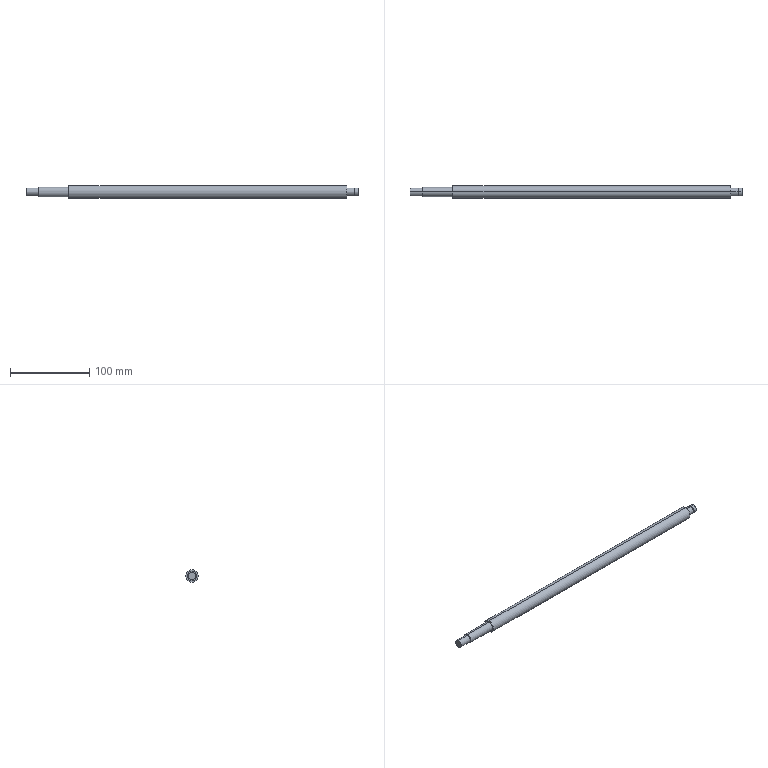Part | STEP file | PN_0033 lead screw 16-5T3 | 1 solid | 19 faces | box 418 x 16 x 16 mm | volume 77018 mm3 | cylinder 12 | plane 7 | commonest cylinder face diameters 10 x6 9.6 x2 12 x2 16 x2
STEP:
#1=CARTESIAN_POINT('',(0.,0.,0.));
#2=DIRECTION('',(0.,0.,1.));
#3=DIRECTION('',(1.,0.,0.));
#4=AXIS2_PLACEMENT_3D('',#1,#2,#3);
#5=CARTESIAN_POINT('',(-3.85,0.,5.));
#6=VERTEX_POINT('',#5);
#7=CARTESIAN_POINT('',(-3.85,0.,-5.));
#8=VERTEX_POINT('',#7);
#9=CARTESIAN_POINT('',(-3.85,0.,0.));
#10=DIRECTION('',(-1.,0.,0.));
#11=DIRECTION('',(0.,0.,-1.));
#12=AXIS2_PLACEMENT_3D('',#9,#10,#11);
#13=CIRCLE('',#12,5.);
#14=CARTESIAN_POINT('',(0.,0.,0.));
#15=DIRECTION('',(1.,0.,0.));
#16=DIRECTION('',(0.,0.,-1.));
#17=AXIS2_PLACEMENT_3D('',#14,#15,#16);
#18=CYLINDRICAL_SURFACE('',#17,5.);
#19=CARTESIAN_POINT('',(6.283,-3.85));
#20=DIRECTION('',(-1.,0.));
#21=VECTOR('',#20,1.);
#22=LINE('',#19,#21);
#23=(GEOMETRIC_REPRESENTATION_CONTEXT(2)PARAMETRIC_REPRESENTATION_CONTEXT()REPRESENTATION_CONTEXT('',''));
#24=DEFINITIONAL_REPRESENTATION('',(#22),#23);
#25=PCURVE('',#18,#24);
#26=CARTESIAN_POINT('',(-3.85,0.,-10.353));
#27=DIRECTION('',(1.,0.,0.));
#28=DIRECTION('',(0.,0.,-1.));
#29=AXIS2_PLACEMENT_3D('',#26,#27,#28);
#30=PLANE('',#29);
#31=CARTESIAN_POINT('',(-5.353,0.));
#32=CARTESIAN_POINT('',(-5.353,-8.66));
#33=CARTESIAN_POINT('',(-12.853,-4.33));
#34=CARTESIAN_POINT('',(-20.353,0.));
#35=CARTESIAN_POINT('',(-12.853,4.33));
#36=CARTESIAN_POINT('',(-5.353,8.66));
#37=CARTESIAN_POINT('',(-5.353,0.));
#38=(BOUNDED_CURVE()B_SPLINE_CURVE(2,(#31,#32,#33,#34,#35,#36,#37),.UNSPECIFIED.,.T.,.F.)B_SPLINE_CURVE_WITH_KNOTS((1,2,2,2,2,1),(-2.094,0.,2.094,4.189,6.283,8.378),.UNSPECIFIED.)CURVE()GEOMETRIC_REPRESENTATION_ITEM()RATIONAL_B_SPLINE_CURVE((1.,0.5,1.,0.5,1.,0.5,1.))REPRESENTATION_ITEM(''));
#39=(GEOMETRIC_REPRESENTATION_CONTEXT(2)PARAMETRIC_REPRESENTATION_CONTEXT()REPRESENTATION_CONTEXT('',''));
#40=DEFINITIONAL_REPRESENTATION('',(#38),#39);
#41=PCURVE('',#30,#40);
#42=SURFACE_CURVE('',#13,(#25,#41),.PCURVE_S1.);
#43=EDGE_CURVE('',#6,#8,#42,.T.);
#44=ORIENTED_EDGE('',*,*,#43,.F.);
#45=CARTESIAN_POINT('',(0.,0.,5.));
#46=VERTEX_POINT('',#45);
#47=CARTESIAN_POINT('',(0.,0.,5.));
#48=DIRECTION('',(1.,0.,0.));
#49=VECTOR('',#48,1.);
#50=LINE('',#47,#49);
#51=CARTESIAN_POINT('',(3.142,0.));
#52=DIRECTION('',(0.,1.));
#53=VECTOR('',#52,1.);
#54=LINE('',#51,#53);
#55=(GEOMETRIC_REPRESENTATION_CONTEXT(2)PARAMETRIC_REPRESENTATION_CONTEXT()REPRESENTATION_CONTEXT('',''));
#56=DEFINITIONAL_REPRESENTATION('',(#54),#55);
#57=PCURVE('',#18,#56);
#58=CARTESIAN_POINT('',(0.,0.,0.));
#59=DIRECTION('',(1.,0.,0.));
#60=DIRECTION('',(0.,0.,-1.));
#61=AXIS2_PLACEMENT_3D('',#58,#59,#60);
#62=CYLINDRICAL_SURFACE('',#61,5.);
#63=CARTESIAN_POINT('',(3.142,0.));
#64=DIRECTION('',(0.,1.));
#65=VECTOR('',#64,1.);
#66=LINE('',#63,#65);
#67=(GEOMETRIC_REPRESENTATION_CONTEXT(2)PARAMETRIC_REPRESENTATION_CONTEXT()REPRESENTATION_CONTEXT('',''));
#68=DEFINITIONAL_REPRESENTATION('',(#66),#67);
#69=PCURVE('',#62,#68);
#70=SURFACE_CURVE('',#50,(#57,#69),.PCURVE_S1.);
#71=EDGE_CURVE('',#6,#46,#70,.T.);
#72=ORIENTED_EDGE('',*,*,#71,.T.);
#73=CARTESIAN_POINT('',(0.,0.,-5.));
#74=VERTEX_POINT('',#73);
#75=CARTESIAN_POINT('',(0.,0.,0.));
#76=DIRECTION('',(1.,0.,0.));
#77=DIRECTION('',(0.,0.,-1.));
#78=AXIS2_PLACEMENT_3D('',#75,#76,#77);
#79=CIRCLE('',#78,5.);
#80=CARTESIAN_POINT('',(0.,0.));
#81=DIRECTION('',(1.,0.));
#82=VECTOR('',#81,1.);
#83=LINE('',#80,#82);
#84=(GEOMETRIC_REPRESENTATION_CONTEXT(2)PARAMETRIC_REPRESENTATION_CONTEXT()REPRESENTATION_CONTEXT('',''));
#85=DEFINITIONAL_REPRESENTATION('',(#83),#84);
#86=PCURVE('',#18,#85);
#87=CARTESIAN_POINT('',(0.,0.,0.));
#88=DIRECTION('',(1.,0.,0.));
#89=DIRECTION('',(0.,0.,-1.));
#90=AXIS2_PLACEMENT_3D('',#87,#88,#89);
#91=PLANE('',#90);
#92=CARTESIAN_POINT('',(0.,0.));
#93=DIRECTION('',(1.,0.));
#94=AXIS2_PLACEMENT_2D('',#92,#93);
#95=CIRCLE('',#94,5.);
#96=(GEOMETRIC_REPRESENTATION_CONTEXT(2)PARAMETRIC_REPRESENTATION_CONTEXT()REPRESENTATION_CONTEXT('',''));
#97=DEFINITIONAL_REPRESENTATION('',(#95),#96);
#98=PCURVE('',#91,#97);
#99=SURFACE_CURVE('',#79,(#86,#98),.PCURVE_S1.);
#100=EDGE_CURVE('',#74,#46,#99,.T.);
#101=ORIENTED_EDGE('',*,*,#100,.F.);
#102=CARTESIAN_POINT('',(0.,0.,-5.));
#103=DIRECTION('',(1.,0.,0.));
#104=VECTOR('',#103,1.);
#105=LINE('',#102,#104);
#106=CARTESIAN_POINT('',(0.,0.));
#107=DIRECTION('',(0.,1.));
#108=VECTOR('',#107,1.);
#109=LINE('',#106,#108);
#110=(GEOMETRIC_REPRESENTATION_CONTEXT(2)PARAMETRIC_REPRESENTATION_CONTEXT()REPRESENTATION_CONTEXT('',''));
#111=DEFINITIONAL_REPRESENTATION('',(#109),#110);
#112=PCURVE('',#18,#111);
#113=CARTESIAN_POINT('',(6.283,0.));
#114=DIRECTION('',(0.,1.));
#115=VECTOR('',#114,1.);
#116=LINE('',#113,#115);
#117=(GEOMETRIC_REPRESENTATION_CONTEXT(2)PARAMETRIC_REPRESENTATION_CONTEXT()REPRESENTATION_CONTEXT('',''));
#118=DEFINITIONAL_REPRESENTATION('',(#116),#117);
#119=PCURVE('',#62,#118);
#120=SURFACE_CURVE('',#105,(#112,#119),.PCURVE_S1.);
#121=EDGE_CURVE('',#8,#74,#120,.T.);
#122=ORIENTED_EDGE('',*,*,#121,.F.);
#123=EDGE_LOOP('',(#44,#72,#101,#122));
#124=FACE_BOUND('',#123,.T.);
#125=ADVANCED_FACE('',(#124),#18,.T.);
#126=CARTESIAN_POINT('',(-5.,0.,-4.8));
#127=VERTEX_POINT('',#126);
#128=CARTESIAN_POINT('',(-5.,0.,4.8));
#129=VERTEX_POINT('',#128);
#130=CARTESIAN_POINT('',(-5.,0.,0.));
#131=DIRECTION('',(1.,0.,0.));
#132=DIRECTION('',(0.,0.,-1.));
#133=AXIS2_PLACEMENT_3D('',#130,#131,#132);
#134=CIRCLE('',#133,4.8);
#135=CARTESIAN_POINT('',(0.,0.,0.));
#136=DIRECTION('',(1.,0.,0.));
#137=DIRECTION('',(0.,0.,-1.));
#138=AXIS2_PLACEMENT_3D('',#135,#136,#137);
#139=CYLINDRICAL_SURFACE('',#138,4.8);
#140=CARTESIAN_POINT('',(0.,-5.));
#141=DIRECTION('',(1.,0.));
#142=VECTOR('',#141,1.);
#143=LINE('',#140,#142);
#144=(GEOMETRIC_REPRESENTATION_CONTEXT(2)PARAMETRIC_REPRESENTATION_CONTEXT()REPRESENTATION_CONTEXT('',''));
#145=DEFINITIONAL_REPRESENTATION('',(#143),#144);
#146=PCURVE('',#139,#145);
#147=CARTESIAN_POINT('',(-5.,0.,-10.353));
#148=DIRECTION('',(-1.,0.,0.));
#149=DIRECTION('',(0.,0.,1.));
#150=AXIS2_PLACEMENT_3D('',#147,#148,#149);
#151=PLANE('',#150);
#152=CARTESIAN_POINT('',(5.553,0.));
#153=CARTESIAN_POINT('',(5.553,8.314));
#154=CARTESIAN_POINT('',(12.753,4.157));
#155=CARTESIAN_POINT('',(19.953,0.));
#156=CARTESIAN_POINT('',(12.753,-4.157));
#157=CARTESIAN_POINT('',(5.553,-8.314));
#158=CARTESIAN_POINT('',(5.553,0.));
#159=(BOUNDED_CURVE()B_SPLINE_CURVE(2,(#152,#153,#154,#155,#156,#157,#158),.UNSPECIFIED.,.T.,.F.)B_SPLINE_CURVE_WITH_KNOTS((1,2,2,2,2,1),(-2.094,0.,2.094,4.189,6.283,8.378),.UNSPECIFIED.)CURVE()GEOMETRIC_REPRESENTATION_ITEM()RATIONAL_B_SPLINE_CURVE((1.,0.5,1.,0.5,1.,0.5,1.))REPRESENTATION_ITEM(''));
#160=(GEOMETRIC_REPRESENTATION_CONTEXT(2)PARAMETRIC_REPRESENTATION_CONTEXT()REPRESENTATION_CONTEXT('',''));
#161=DEFINITIONAL_REPRESENTATION('',(#159),#160);
#162=PCURVE('',#151,#161);
#163=SURFACE_CURVE('',#134,(#146,#162),.PCURVE_S1.);
#164=EDGE_CURVE('',#127,#129,#163,.T.);
#165=ORIENTED_EDGE('',*,*,#164,.T.);
#166=CARTESIAN_POINT('',(-3.85,0.,4.8));
#167=VERTEX_POINT('',#166);
#168=CARTESIAN_POINT('',(0.,0.,4.8));
#169=DIRECTION('',(1.,0.,0.));
#170=VECTOR('',#169,1.);
#171=LINE('',#168,#170);
#172=CARTESIAN_POINT('',(3.142,0.));
#173=DIRECTION('',(0.,1.));
#174=VECTOR('',#173,1.);
#175=LINE('',#172,#174);
#176=(GEOMETRIC_REPRESENTATION_CONTEXT(2)PARAMETRIC_REPRESENTATION_CONTEXT()REPRESENTATION_CONTEXT('',''));
#177=DEFINITIONAL_REPRESENTATION('',(#175),#176);
#178=PCURVE('',#139,#177);
#179=CARTESIAN_POINT('',(0.,0.,0.));
#180=DIRECTION('',(1.,0.,0.));
#181=DIRECTION('',(0.,0.,-1.));
#182=AXIS2_PLACEMENT_3D('',#179,#180,#181);
#183=CYLINDRICAL_SURFACE('',#182,4.8);
#184=CARTESIAN_POINT('',(3.142,0.));
#185=DIRECTION('',(0.,1.));
#186=VECTOR('',#185,1.);
#187=LINE('',#184,#186);
#188=(GEOMETRIC_REPRESENTATION_CONTEXT(2)PARAMETRIC_REPRESENTATION_CONTEXT()REPRESENTATION_CONTEXT('',''));
#189=DEFINITIONAL_REPRESENTATION('',(#187),#188);
#190=PCURVE('',#183,#189);
#191=SURFACE_CURVE('',#171,(#178,#190),.PCURVE_S1.);
#192=EDGE_CURVE('',#129,#167,#191,.T.);
#193=ORIENTED_EDGE('',*,*,#192,.T.);
#194=CARTESIAN_POINT('',(-3.85,0.,-4.8));
#195=VERTEX_POINT('',#194);
#196=CARTESIAN_POINT('',(-3.85,0.,0.));
#197=DIRECTION('',(1.,0.,0.));
#198=DIRECTION('',(0.,0.,-1.));
#199=AXIS2_PLACEMENT_3D('',#196,#197,#198);
#200=CIRCLE('',#199,4.8);
#201=CARTESIAN_POINT('',(0.,-3.85));
#202=DIRECTION('',(1.,0.));
#203=VECTOR('',#202,1.);
#204=LINE('',#201,#203);
#205=(GEOMETRIC_REPRESENTATION_CONTEXT(2)PARAMETRIC_REPRESENTATION_CONTEXT()REPRESENTATION_CONTEXT('',''));
#206=DEFINITIONAL_REPRESENTATION('',(#204),#205);
#207=PCURVE('',#139,#206);
#208=CARTESIAN_POINT('',(-10.353,0.));
#209=DIRECTION('',(1.,0.));
#210=AXIS2_PLACEMENT_2D('',#208,#209);
#211=CIRCLE('',#210,4.8);
#212=(GEOMETRIC_REPRESENTATION_CONTEXT(2)PARAMETRIC_REPRESENTATION_CONTEXT()REPRESENTATION_CONTEXT('',''));
#213=DEFINITIONAL_REPRESENTATION('',(#211),#212);
#214=PCURVE('',#30,#213);
#215=SURFACE_CURVE('',#200,(#207,#214),.PCURVE_S1.);
#216=EDGE_CURVE('',#195,#167,#215,.T.);
#217=ORIENTED_EDGE('',*,*,#216,.F.);
#218=CARTESIAN_POINT('',(0.,0.,-4.8));
#219=DIRECTION('',(1.,0.,0.));
#220=VECTOR('',#219,1.);
#221=LINE('',#218,#220);
#222=CARTESIAN_POINT('',(0.,0.));
#223=DIRECTION('',(0.,1.));
#224=VECTOR('',#223,1.);
#225=LINE('',#222,#224);
#226=(GEOMETRIC_REPRESENTATION_CONTEXT(2)PARAMETRIC_REPRESENTATION_CONTEXT()REPRESENTATION_CONTEXT('',''));
#227=DEFINITIONAL_REPRESENTATION('',(#225),#226);
#228=PCURVE('',#139,#227);
#229=CARTESIAN_POINT('',(6.283,0.));
#230=DIRECTION('',(0.,1.));
#231=VECTOR('',#230,1.);
#232=LINE('',#229,#231);
#233=(GEOMETRIC_REPRESENTATION_CONTEXT(2)PARAMETRIC_REPRESENTATION_CONTEXT()REPRESENTATION_CONTEXT('',''));
#234=DEFINITIONAL_REPRESENTATION('',(#232),#233);
#235=PCURVE('',#183,#234);
#236=SURFACE_CURVE('',#221,(#228,#235),.PCURVE_S1.);
#237=EDGE_CURVE('',#127,#195,#236,.T.);
#238=ORIENTED_EDGE('',*,*,#237,.F.);
#239=EDGE_LOOP('',(#165,#193,#217,#238));
#240=FACE_BOUND('',#239,.T.);
#241=ADVANCED_FACE('',(#240),#139,.T.);
#242=CARTESIAN_POINT('',(-418.,0.,-5.));
#243=VERTEX_POINT('',#242);
#244=CARTESIAN_POINT('',(-418.,0.,5.));
#245=VERTEX_POINT('',#244);
#246=CARTESIAN_POINT('',(-418.,0.,0.));
#247=DIRECTION('',(1.,0.,0.));
#248=DIRECTION('',(0.,0.,-1.));
#249=AXIS2_PLACEMENT_3D('',#246,#247,#248);
#250=CIRCLE('',#249,5.);
#251=CARTESIAN_POINT('',(0.,0.,0.));
#252=DIRECTION('',(1.,0.,0.));
#253=DIRECTION('',(0.,0.,-1.));
#254=AXIS2_PLACEMENT_3D('',#251,#252,#253);
#255=CYLINDRICAL_SURFACE('',#254,5.);
#256=CARTESIAN_POINT('',(0.,-418.));
#257=DIRECTION('',(1.,0.));
#258=VECTOR('',#257,1.);
#259=LINE('',#256,#258);
#260=(GEOMETRIC_REPRESENTATION_CONTEXT(2)PARAMETRIC_REPRESENTATION_CONTEXT()REPRESENTATION_CONTEXT('',''));
#261=DEFINITIONAL_REPRESENTATION('',(#259),#260);
#262=PCURVE('',#255,#261);
#263=CARTESIAN_POINT('',(-418.,5.,0.));
#264=DIRECTION('',(-1.,0.,0.));
#265=DIRECTION('',(0.,0.,1.));
#266=AXIS2_PLACEMENT_3D('',#263,#264,#265);
#267=PLANE('',#266);
#268=CARTESIAN_POINT('',(-5.,-5.));
#269=CARTESIAN_POINT('',(-5.,3.66));
#270=CARTESIAN_POINT('',(2.5,-0.6699));
#271=CARTESIAN_POINT('',(10.,-5.));
#272=CARTESIAN_POINT('',(2.5,-9.33));
#273=CARTESIAN_POINT('',(-5.,-13.66));
#274=CARTESIAN_POINT('',(-5.,-5.));
#275=(BOUNDED_CURVE()B_SPLINE_CURVE(2,(#268,#269,#270,#271,#272,#273,#274),.UNSPECIFIED.,.T.,.F.)B_SPLINE_CURVE_WITH_KNOTS((1,2,2,2,2,1),(-2.094,0.,2.094,4.189,6.283,8.378),.UNSPECIFIED.)CURVE()GEOMETRIC_REPRESENTATION_ITEM()RATIONAL_B_SPLINE_CURVE((1.,0.5,1.,0.5,1.,0.5,1.))REPRESENTATION_ITEM(''));
#276=(GEOMETRIC_REPRESENTATION_CONTEXT(2)PARAMETRIC_REPRESENTATION_CONTEXT()REPRESENTATION_CONTEXT('',''));
#277=DEFINITIONAL_REPRESENTATION('',(#275),#276);
#278=PCURVE('',#267,#277);
#279=SURFACE_CURVE('',#250,(#262,#278),.PCURVE_S1.);
#280=EDGE_CURVE('',#243,#245,#279,.T.);
#281=ORIENTED_EDGE('',*,*,#280,.T.);
#282=CARTESIAN_POINT('',(-402.,0.,5.));
#283=VERTEX_POINT('',#282);
#284=CARTESIAN_POINT('',(0.,0.,5.));
#285=DIRECTION('',(1.,0.,0.));
#286=VECTOR('',#285,1.);
#287=LINE('',#284,#286);
#288=CARTESIAN_POINT('',(3.142,0.));
#289=DIRECTION('',(0.,1.));
#290=VECTOR('',#289,1.);
#291=LINE('',#288,#290);
#292=(GEOMETRIC_REPRESENTATION_CONTEXT(2)PARAMETRIC_REPRESENTATION_CONTEXT()REPRESENTATION_CONTEXT('',''));
#293=DEFINITIONAL_REPRESENTATION('',(#291),#292);
#294=PCURVE('',#255,#293);
#295=CARTESIAN_POINT('',(0.,0.,0.));
#296=DIRECTION('',(1.,0.,0.));
#297=DIRECTION('',(0.,0.,-1.));
#298=AXIS2_PLACEMENT_3D('',#295,#296,#297);
#299=CYLINDRICAL_SURFACE('',#298,5.);
#300=CARTESIAN_POINT('',(3.142,0.));
#301=DIRECTION('',(0.,1.));
#302=VECTOR('',#301,1.);
#303=LINE('',#300,#302);
#304=(GEOMETRIC_REPRESENTATION_CONTEXT(2)PARAMETRIC_REPRESENTATION_CONTEXT()REPRESENTATION_CONTEXT('',''));
#305=DEFINITIONAL_REPRESENTATION('',(#303),#304);
#306=PCURVE('',#299,#305);
#307=SURFACE_CURVE('',#287,(#294,#306),.PCURVE_S1.);
#308=EDGE_CURVE('',#245,#283,#307,.T.);
#309=ORIENTED_EDGE('',*,*,#308,.T.);
#310=CARTESIAN_POINT('',(-402.,0.,-5.));
#311=VERTEX_POINT('',#310);
#312=CARTESIAN_POINT('',(-402.,0.,0.));
#313=DIRECTION('',(1.,0.,0.));
#314=DIRECTION('',(0.,0.,-1.));
#315=AXIS2_PLACEMENT_3D('',#312,#313,#314);
#316=CIRCLE('',#315,5.);
#317=CARTESIAN_POINT('',(0.,-402.));
#318=DIRECTION('',(1.,0.));
#319=VECTOR('',#318,1.);
#320=LINE('',#317,#319);
#321=(GEOMETRIC_REPRESENTATION_CONTEXT(2)PARAMETRIC_REPRESENTATION_CONTEXT()REPRESENTATION_CONTEXT('',''));
#322=DEFINITIONAL_REPRESENTATION('',(#320),#321);
#323=PCURVE('',#255,#322);
#324=CARTESIAN_POINT('',(-402.,6.,0.));
#325=DIRECTION('',(-1.,0.,0.));
#326=DIRECTION('',(0.,0.,1.));
#327=AXIS2_PLACEMENT_3D('',#324,#325,#326);
#328=PLANE('',#327);
#329=CARTESIAN_POINT('',(-5.,-6.));
#330=CARTESIAN_POINT('',(-5.,2.66));
#331=CARTESIAN_POINT('',(2.5,-1.67));
#332=CARTESIAN_POINT('',(10.,-6.));
#333=CARTESIAN_POINT('',(2.5,-10.33));
#334=CARTESIAN_POINT('',(-5.,-14.66));
#335=CARTESIAN_POINT('',(-5.,-6.));
#336=(BOUNDED_CURVE()B_SPLINE_CURVE(2,(#329,#330,#331,#332,#333,#334,#335),.UNSPECIFIED.,.T.,.F.)B_SPLINE_CURVE_WITH_KNOTS((1,2,2,2,2,1),(-2.094,0.,2.094,4.189,6.283,8.378),.UNSPECIFIED.)CURVE()GEOMETRIC_REPRESENTATION_ITEM()RATIONAL_B_SPLINE_CURVE((1.,0.5,1.,0.5,1.,0.5,1.))REPRESENTATION_ITEM(''));
#337=(GEOMETRIC_REPRESENTATION_CONTEXT(2)PARAMETRIC_REPRESENTATION_CONTEXT()REPRESENTATION_CONTEXT('',''));
#338=DEFINITIONAL_REPRESENTATION('',(#336),#337);
#339=PCURVE('',#328,#338);
#340=SURFACE_CURVE('',#316,(#323,#339),.PCURVE_S1.);
#341=EDGE_CURVE('',#311,#283,#340,.T.);
#342=ORIENTED_EDGE('',*,*,#341,.F.);
#343=CARTESIAN_POINT('',(0.,0.,-5.));
#344=DIRECTION('',(1.,0.,0.));
#345=VECTOR('',#344,1.);
#346=LINE('',#343,#345);
#347=CARTESIAN_POINT('',(0.,0.));
#348=DIRECTION('',(0.,1.));
#349=VECTOR('',#348,1.);
#350=LINE('',#347,#349);
#351=(GEOMETRIC_REPRESENTATION_CONTEXT(2)PARAMETRIC_REPRESENTATION_CONTEXT()REPRESENTATION_CONTEXT('',''));
#352=DEFINITIONAL_REPRESENTATION('',(#350),#351);
#353=PCURVE('',#255,#352);
#354=CARTESIAN_POINT('',(6.283,0.));
#355=DIRECTION('',(0.,1.));
#356=VECTOR('',#355,1.);
#357=LINE('',#354,#356);
#358=(GEOMETRIC_REPRESENTATION_CONTEXT(2)PARAMETRIC_REPRESENTATION_CONTEXT()REPRESENTATION_CONTEXT('',''));
#359=DEFINITIONAL_REPRESENTATION('',(#357),#358);
#360=PCURVE('',#299,#359);
#361=SURFACE_CURVE('',#346,(#353,#360),.PCURVE_S1.);
#362=EDGE_CURVE('',#243,#311,#361,.T.);
#363=ORIENTED_EDGE('',*,*,#362,.F.);
#364=EDGE_LOOP('',(#281,#309,#342,#363));
#365=FACE_BOUND('',#364,.T.);
#366=ADVANCED_FACE('',(#365),#255,.T.);
#367=CARTESIAN_POINT('',(-402.,0.,-6.));
#368=VERTEX_POINT('',#367);
#369=CARTESIAN_POINT('',(-402.,0.,6.));
#370=VERTEX_POINT('',#369);
#371=CARTESIAN_POINT('',(-402.,0.,0.));
#372=DIRECTION('',(1.,0.,0.));
#373=DIRECTION('',(0.,0.,-1.));
#374=AXIS2_PLACEMENT_3D('',#371,#372,#373);
#375=CIRCLE('',#374,6.);
#376=CARTESIAN_POINT('',(0.,0.,0.));
#377=DIRECTION('',(1.,0.,0.));
#378=DIRECTION('',(0.,0.,-1.));
#379=AXIS2_PLACEMENT_3D('',#376,#377,#378);
#380=CYLINDRICAL_SURFACE('',#379,6.);
#381=CARTESIAN_POINT('',(0.,-402.));
#382=DIRECTION('',(1.,0.));
#383=VECTOR('',#382,1.);
#384=LINE('',#381,#383);
#385=(GEOMETRIC_REPRESENTATION_CONTEXT(2)PARAMETRIC_REPRESENTATION_CONTEXT()REPRESENTATION_CONTEXT('',''));
#386=DEFINITIONAL_REPRESENTATION('',(#384),#385);
#387=PCURVE('',#380,#386);
#388=CARTESIAN_POINT('',(-6.,-6.));
#389=CARTESIAN_POINT('',(-6.,4.392));
#390=CARTESIAN_POINT('',(3.,-0.8038));
#391=CARTESIAN_POINT('',(12.,-6.));
#392=CARTESIAN_POINT('',(3.,-11.196));
#393=CARTESIAN_POINT('',(-6.,-16.392));
#394=CARTESIAN_POINT('',(-6.,-6.));
#395=(BOUNDED_CURVE()B_SPLINE_CURVE(2,(#388,#389,#390,#391,#392,#393,#394),.UNSPECIFIED.,.T.,.F.)B_SPLINE_CURVE_WITH_KNOTS((1,2,2,2,2,1),(-2.094,0.,2.094,4.189,6.283,8.378),.UNSPECIFIED.)CURVE()GEOMETRIC_REPRESENTATION_ITEM()RATIONAL_B_SPLINE_CURVE((1.,0.5,1.,0.5,1.,0.5,1.))REPRESENTATION_ITEM(''));
#396=(GEOMETRIC_REPRESENTATION_CONTEXT(2)PARAMETRIC_REPRESENTATION_CONTEXT()REPRESENTATION_CONTEXT('',''));
#397=DEFINITIONAL_REPRESENTATION('',(#395),#396);
#398=PCURVE('',#328,#397);
#399=SURFACE_CURVE('',#375,(#387,#398),.PCURVE_S1.);
#400=EDGE_CURVE('',#368,#370,#399,.T.);
#401=ORIENTED_EDGE('',*,*,#400,.T.);
#402=CARTESIAN_POINT('',(-364.,0.,6.));
#403=VERTEX_POINT('',#402);
#404=CARTESIAN_POINT('',(0.,0.,6.));
#405=DIRECTION('',(1.,0.,0.));
#406=VECTOR('',#405,1.);
#407=LINE('',#404,#406);
#408=CARTESIAN_POINT('',(3.142,0.));
#409=DIRECTION('',(0.,1.));
#410=VECTOR('',#409,1.);
#411=LINE('',#408,#410);
#412=(GEOMETRIC_REPRESENTATION_CONTEXT(2)PARAMETRIC_REPRESENTATION_CONTEXT()REPRESENTATION_CONTEXT('',''));
#413=DEFINITIONAL_REPRESENTATION('',(#411),#412);
#414=PCURVE('',#380,#413);
#415=CARTESIAN_POINT('',(0.,0.,0.));
#416=DIRECTION('',(1.,0.,0.));
#417=DIRECTION('',(0.,0.,-1.));
#418=AXIS2_PLACEMENT_3D('',#415,#416,#417);
#419=CYLINDRICAL_SURFACE('',#418,6.);
#420=CARTESIAN_POINT('',(3.142,0.));
#421=DIRECTION('',(0.,1.));
#422=VECTOR('',#421,1.);
#423=LINE('',#420,#422);
#424=(GEOMETRIC_REPRESENTATION_CONTEXT(2)PARAMETRIC_REPRESENTATION_CONTEXT()REPRESENTATION_CONTEXT('',''));
#425=DEFINITIONAL_REPRESENTATION('',(#423),#424);
#426=PCURVE('',#419,#425);
#427=SURFACE_CURVE('',#407,(#414,#426),.PCURVE_S1.);
#428=EDGE_CURVE('',#370,#403,#427,.T.);
#429=ORIENTED_EDGE('',*,*,#428,.T.);
#430=CARTESIAN_POINT('',(-364.,0.,-6.));
#431=VERTEX_POINT('',#430);
#432=CARTESIAN_POINT('',(-364.,0.,0.));
#433=DIRECTION('',(1.,0.,0.));
#434=DIRECTION('',(0.,0.,-1.));
#435=AXIS2_PLACEMENT_3D('',#432,#433,#434);
#436=CIRCLE('',#435,6.);
#437=CARTESIAN_POINT('',(0.,-364.));
#438=DIRECTION('',(1.,0.));
#439=VECTOR('',#438,1.);
#440=LINE('',#437,#439);
#441=(GEOMETRIC_REPRESENTATION_CONTEXT(2)PARAMETRIC_REPRESENTATION_CONTEXT()REPRESENTATION_CONTEXT('',''));
#442=DEFINITIONAL_REPRESENTATION('',(#440),#441);
#443=PCURVE('',#380,#442);
#444=CARTESIAN_POINT('',(-364.,8.,0.));
#445=DIRECTION('',(-1.,0.,0.));
#446=DIRECTION('',(0.,0.,1.));
#447=AXIS2_PLACEMENT_3D('',#444,#445,#446);
#448=PLANE('',#447);
#449=CARTESIAN_POINT('',(-6.,-8.));
#450=CARTESIAN_POINT('',(-6.,2.392));
#451=CARTESIAN_POINT('',(3.,-2.804));
#452=CARTESIAN_POINT('',(12.,-8.));
#453=CARTESIAN_POINT('',(3.,-13.196));
#454=CARTESIAN_POINT('',(-6.,-18.392));
#455=CARTESIAN_POINT('',(-6.,-8.));
#456=(BOUNDED_CURVE()B_SPLINE_CURVE(2,(#449,#450,#451,#452,#453,#454,#455),.UNSPECIFIED.,.T.,.F.)B_SPLINE_CURVE_WITH_KNOTS((1,2,2,2,2,1),(-2.094,0.,2.094,4.189,6.283,8.378),.UNSPECIFIED.)CURVE()GEOMETRIC_REPRESENTATION_ITEM()RATIONAL_B_SPLINE_CURVE((1.,0.5,1.,0.5,1.,0.5,1.))REPRESENTATION_ITEM(''));
#457=(GEOMETRIC_REPRESENTATION_CONTEXT(2)PARAMETRIC_REPRESENTATION_CONTEXT()REPRESENTATION_CONTEXT('',''));
#458=DEFINITIONAL_REPRESENTATION('',(#456),#457);
#459=PCURVE('',#448,#458);
#460=SURFACE_CURVE('',#436,(#443,#459),.PCURVE_S1.);
#461=EDGE_CURVE('',#431,#403,#460,.T.);
#462=ORIENTED_EDGE('',*,*,#461,.F.);
#463=CARTESIAN_POINT('',(0.,0.,-6.));
#464=DIRECTION('',(1.,0.,0.));
#465=VECTOR('',#464,1.);
#466=LINE('',#463,#465);
#467=CARTESIAN_POINT('',(0.,0.));
#468=DIRECTION('',(0.,1.));
#469=VECTOR('',#468,1.);
#470=LINE('',#467,#469);
#471=(GEOMETRIC_REPRESENTATION_CONTEXT(2)PARAMETRIC_REPRESENTATION_CONTEXT()REPRESENTATION_CONTEXT('',''));
#472=DEFINITIONAL_REPRESENTATION('',(#470),#471);
#473=PCURVE('',#380,#472);
#474=CARTESIAN_POINT('',(6.283,0.));
#475=DIRECTION('',(0.,1.));
#476=VECTOR('',#475,1.);
#477=LINE('',#474,#476);
#478=(GEOMETRIC_REPRESENTATION_CONTEXT(2)PARAMETRIC_REPRESENTATION_CONTEXT()REPRESENTATION_CONTEXT('',''));
#479=DEFINITIONAL_REPRESENTATION('',(#477),#478);
#480=PCURVE('',#419,#479);
#481=SURFACE_CURVE('',#466,(#473,#480),.PCURVE_S1.);
#482=EDGE_CURVE('',#368,#431,#481,.T.);
#483=ORIENTED_EDGE('',*,*,#482,.F.);
#484=EDGE_LOOP('',(#401,#429,#462,#483));
#485=FACE_BOUND('',#484,.T.);
#486=ADVANCED_FACE('',(#485),#380,.T.);
#487=CARTESIAN_POINT('',(-364.,0.,-8.));
#488=VERTEX_POINT('',#487);
#489=CARTESIAN_POINT('',(-364.,0.,8.));
#490=VERTEX_POINT('',#489);
#491=CARTESIAN_POINT('',(-364.,0.,0.));
#492=DIRECTION('',(1.,0.,0.));
#493=DIRECTION('',(0.,0.,-1.));
#494=AXIS2_PLACEMENT_3D('',#491,#492,#493);
#495=CIRCLE('',#494,8.);
#496=CARTESIAN_POINT('',(0.,0.,0.));
#497=DIRECTION('',(1.,0.,0.));
#498=DIRECTION('',(0.,0.,-1.));
#499=AXIS2_PLACEMENT_3D('',#496,#497,#498);
#500=CYLINDRICAL_SURFACE('',#499,8.);
#501=CARTESIAN_POINT('',(0.,-364.));
#502=DIRECTION('',(1.,0.));
#503=VECTOR('',#502,1.);
#504=LINE('',#501,#503);
#505=(GEOMETRIC_REPRESENTATION_CONTEXT(2)PARAMETRIC_REPRESENTATION_CONTEXT()REPRESENTATION_CONTEXT('',''));
#506=DEFINITIONAL_REPRESENTATION('',(#504),#505);
#507=PCURVE('',#500,#506);
#508=CARTESIAN_POINT('',(-8.,-8.));
#509=CARTESIAN_POINT('',(-8.,5.856));
#510=CARTESIAN_POINT('',(4.,-1.072));
#511=CARTESIAN_POINT('',(16.,-8.));
#512=CARTESIAN_POINT('',(4.,-14.928));
#513=CARTESIAN_POINT('',(-8.,-21.856));
#514=CARTESIAN_POINT('',(-8.,-8.));
#515=(BOUNDED_CURVE()B_SPLINE_CURVE(2,(#508,#509,#510,#511,#512,#513,#514),.UNSPECIFIED.,.T.,.F.)B_SPLINE_CURVE_WITH_KNOTS((1,2,2,2,2,1),(-2.094,0.,2.094,4.189,6.283,8.378),.UNSPECIFIED.)CURVE()GEOMETRIC_REPRESENTATION_ITEM()RATIONAL_B_SPLINE_CURVE((1.,0.5,1.,0.5,1.,0.5,1.))REPRESENTATION_ITEM(''));
#516=(GEOMETRIC_REPRESENTATION_CONTEXT(2)PARAMETRIC_REPRESENTATION_CONTEXT()REPRESENTATION_CONTEXT('',''));
#517=DEFINITIONAL_REPRESENTATION('',(#515),#516);
#518=PCURVE('',#448,#517);
#519=SURFACE_CURVE('',#495,(#507,#518),.PCURVE_S1.);
#520=EDGE_CURVE('',#488,#490,#519,.T.);
#521=ORIENTED_EDGE('',*,*,#520,.T.);
#522=CARTESIAN_POINT('',(-14.,0.,8.));
#523=VERTEX_POINT('',#522);
#524=CARTESIAN_POINT('',(0.,0.,8.));
#525=DIRECTION('',(1.,0.,0.));
#526=VECTOR('',#525,1.);
#527=LINE('',#524,#526);
#528=CARTESIAN_POINT('',(3.142,0.));
#529=DIRECTION('',(0.,1.));
#530=VECTOR('',#529,1.);
#531=LINE('',#528,#530);
#532=(GEOMETRIC_REPRESENTATION_CONTEXT(2)PARAMETRIC_REPRESENTATION_CONTEXT()REPRESENTATION_CONTEXT('',''));
#533=DEFINITIONAL_REPRESENTATION('',(#531),#532);
#534=PCURVE('',#500,#533);
#535=CARTESIAN_POINT('',(0.,0.,0.));
#536=DIRECTION('',(1.,0.,0.));
#537=DIRECTION('',(0.,0.,-1.));
#538=AXIS2_PLACEMENT_3D('',#535,#536,#537);
#539=CYLINDRICAL_SURFACE('',#538,8.);
#540=CARTESIAN_POINT('',(3.142,0.));
#541=DIRECTION('',(0.,1.));
#542=VECTOR('',#541,1.);
#543=LINE('',#540,#542);
#544=(GEOMETRIC_REPRESENTATION_CONTEXT(2)PARAMETRIC_REPRESENTATION_CONTEXT()REPRESENTATION_CONTEXT('',''));
#545=DEFINITIONAL_REPRESENTATION('',(#543),#544);
#546=PCURVE('',#539,#545);
#547=SURFACE_CURVE('',#527,(#534,#546),.PCURVE_S1.);
#548=EDGE_CURVE('',#490,#523,#547,.T.);
#549=ORIENTED_EDGE('',*,*,#548,.T.);
#550=CARTESIAN_POINT('',(-14.,0.,-8.));
#551=VERTEX_POINT('',#550);
#552=CARTESIAN_POINT('',(-14.,0.,0.));
#553=DIRECTION('',(1.,0.,0.));
#554=DIRECTION('',(0.,0.,-1.));
#555=AXIS2_PLACEMENT_3D('',#552,#553,#554);
#556=CIRCLE('',#555,8.);
#557=CARTESIAN_POINT('',(0.,-14.));
#558=DIRECTION('',(1.,0.));
#559=VECTOR('',#558,1.);
#560=LINE('',#557,#559);
#561=(GEOMETRIC_REPRESENTATION_CONTEXT(2)PARAMETRIC_REPRESENTATION_CONTEXT()REPRESENTATION_CONTEXT('',''));
#562=DEFINITIONAL_REPRESENTATION('',(#560),#561);
#563=PCURVE('',#500,#562);
#564=CARTESIAN_POINT('',(-14.,5.,0.));
#565=DIRECTION('',(1.,0.,0.));
#566=DIRECTION('',(0.,0.,-1.));
#567=AXIS2_PLACEMENT_3D('',#564,#565,#566);
#568=PLANE('',#567);
#569=CARTESIAN_POINT('',(0.,-5.));
#570=DIRECTION('',(1.,0.));
#571=AXIS2_PLACEMENT_2D('',#569,#570);
#572=CIRCLE('',#571,8.);
#573=(GEOMETRIC_REPRESENTATION_CONTEXT(2)PARAMETRIC_REPRESENTATION_CONTEXT()REPRESENTATION_CONTEXT('',''));
#574=DEFINITIONAL_REPRESENTATION('',(#572),#573);
#575=PCURVE('',#568,#574);
#576=SURFACE_CURVE('',#556,(#563,#575),.PCURVE_S1.);
#577=EDGE_CURVE('',#551,#523,#576,.T.);
#578=ORIENTED_EDGE('',*,*,#577,.F.);
#579=CARTESIAN_POINT('',(0.,0.,-8.));
#580=DIRECTION('',(1.,0.,0.));
#581=VECTOR('',#580,1.);
#582=LINE('',#579,#581);
#583=CARTESIAN_POINT('',(0.,0.));
#584=DIRECTION('',(0.,1.));
#585=VECTOR('',#584,1.);
#586=LINE('',#583,#585);
#587=(GEOMETRIC_REPRESENTATION_CONTEXT(2)PARAMETRIC_REPRESENTATION_CONTEXT()REPRESENTATION_CONTEXT('',''));
#588=DEFINITIONAL_REPRESENTATION('',(#586),#587);
#589=PCURVE('',#500,#588);
#590=CARTESIAN_POINT('',(6.283,0.));
#591=DIRECTION('',(0.,1.));
#592=VECTOR('',#591,1.);
#593=LINE('',#590,#592);
#594=(GEOMETRIC_REPRESENTATION_CONTEXT(2)PARAMETRIC_REPRESENTATION_CONTEXT()REPRESENTATION_CONTEXT('',''));
#595=DEFINITIONAL_REPRESENTATION('',(#593),#594);
#596=PCURVE('',#539,#595);
#597=SURFACE_CURVE('',#582,(#589,#596),.PCURVE_S1.);
#598=EDGE_CURVE('',#488,#551,#597,.T.);
#599=ORIENTED_EDGE('',*,*,#598,.F.);
#600=EDGE_LOOP('',(#521,#549,#578,#599));
#601=FACE_BOUND('',#600,.T.);
#602=ADVANCED_FACE('',(#601),#500,.T.);
#603=CARTESIAN_POINT('',(-14.,0.,-5.));
#604=VERTEX_POINT('',#603);
#605=CARTESIAN_POINT('',(-14.,0.,5.));
#606=VERTEX_POINT('',#605);
#607=CARTESIAN_POINT('',(-14.,0.,0.));
#608=DIRECTION('',(1.,0.,0.));
#609=DIRECTION('',(0.,0.,-1.));
#610=AXIS2_PLACEMENT_3D('',#607,#608,#609);
#611=CIRCLE('',#610,5.);
#612=CARTESIAN_POINT('',(0.,0.,0.));
#613=DIRECTION('',(1.,0.,0.));
#614=DIRECTION('',(0.,0.,-1.));
#615=AXIS2_PLACEMENT_3D('',#612,#613,#614);
#616=CYLINDRICAL_SURFACE('',#615,5.);
#617=CARTESIAN_POINT('',(0.,-14.));
#618=DIRECTION('',(1.,0.));
#619=VECTOR('',#618,1.);
#620=LINE('',#617,#619);
#621=(GEOMETRIC_REPRESENTATION_CONTEXT(2)PARAMETRIC_REPRESENTATION_CONTEXT()REPRESENTATION_CONTEXT('',''));
#622=DEFINITIONAL_REPRESENTATION('',(#620),#621);
#623=PCURVE('',#616,#622);
#624=CARTESIAN_POINT('',(0.,-5.));
#625=DIRECTION('',(1.,0.));
#626=AXIS2_PLACEMENT_2D('',#624,#625);
#627=CIRCLE('',#626,5.);
#628=(GEOMETRIC_REPRESENTATION_CONTEXT(2)PARAMETRIC_REPRESENTATION_CONTEXT()REPRESENTATION_CONTEXT('',''));
#629=DEFINITIONAL_REPRESENTATION('',(#627),#628);
#630=PCURVE('',#568,#629);
#631=SURFACE_CURVE('',#611,(#623,#630),.PCURVE_S1.);
#632=EDGE_CURVE('',#604,#606,#631,.T.);
#633=ORIENTED_EDGE('',*,*,#632,.T.);
#634=CARTESIAN_POINT('',(-5.,0.,5.));
#635=VERTEX_POINT('',#634);
#636=CARTESIAN_POINT('',(0.,0.,5.));
#637=DIRECTION('',(1.,0.,0.));
#638=VECTOR('',#637,1.);
#639=LINE('',#636,#638);
#640=CARTESIAN_POINT('',(3.142,0.));
#641=DIRECTION('',(0.,1.));
#642=VECTOR('',#641,1.);
#643=LINE('',#640,#642);
#644=(GEOMETRIC_REPRESENTATION_CONTEXT(2)PARAMETRIC_REPRESENTATION_CONTEXT()REPRESENTATION_CONTEXT('',''));
#645=DEFINITIONAL_REPRESENTATION('',(#643),#644);
#646=PCURVE('',#616,#645);
#647=CARTESIAN_POINT('',(0.,0.,0.));
#648=DIRECTION('',(1.,0.,0.));
#649=DIRECTION('',(0.,0.,-1.));
#650=AXIS2_PLACEMENT_3D('',#647,#648,#649);
#651=CYLINDRICAL_SURFACE('',#650,5.);
#652=CARTESIAN_POINT('',(3.142,0.));
#653=DIRECTION('',(0.,1.));
#654=VECTOR('',#653,1.);
#655=LINE('',#652,#654);
#656=(GEOMETRIC_REPRESENTATION_CONTEXT(2)PARAMETRIC_REPRESENTATION_CONTEXT()REPRESENTATION_CONTEXT('',''));
#657=DEFINITIONAL_REPRESENTATION('',(#655),#656);
#658=PCURVE('',#651,#657);
#659=SURFACE_CURVE('',#639,(#646,#658),.PCURVE_S1.);
#660=EDGE_CURVE('',#606,#635,#659,.T.);
#661=ORIENTED_EDGE('',*,*,#660,.T.);
#662=CARTESIAN_POINT('',(-5.,0.,-5.));
#663=VERTEX_POINT('',#662);
#664=CARTESIAN_POINT('',(-5.,0.,0.));
#665=DIRECTION('',(1.,0.,0.));
#666=DIRECTION('',(0.,0.,1.));
#667=AXIS2_PLACEMENT_3D('',#664,#665,#666);
#668=CIRCLE('',#667,5.);
#669=CARTESIAN_POINT('',(-3.142,-5.));
#670=DIRECTION('',(1.,0.));
#671=VECTOR('',#670,1.);
#672=LINE('',#669,#671);
#673=(GEOMETRIC_REPRESENTATION_CONTEXT(2)PARAMETRIC_REPRESENTATION_CONTEXT()REPRESENTATION_CONTEXT('',''));
#674=DEFINITIONAL_REPRESENTATION('',(#672),#673);
#675=PCURVE('',#616,#674);
#676=CARTESIAN_POINT('',(15.353,0.));
#677=CARTESIAN_POINT('',(15.353,-8.66));
#678=CARTESIAN_POINT('',(7.853,-4.33));
#679=CARTESIAN_POINT('',(0.3531,0.));
#680=CARTESIAN_POINT('',(7.853,4.33));
#681=CARTESIAN_POINT('',(15.353,8.66));
#682=CARTESIAN_POINT('',(15.353,0.));
#683=(BOUNDED_CURVE()B_SPLINE_CURVE(2,(#676,#677,#678,#679,#680,#681,#682),.UNSPECIFIED.,.T.,.F.)B_SPLINE_CURVE_WITH_KNOTS((1,2,2,2,2,1),(-2.094,0.,2.094,4.189,6.283,8.378),.UNSPECIFIED.)CURVE()GEOMETRIC_REPRESENTATION_ITEM()RATIONAL_B_SPLINE_CURVE((1.,0.5,1.,0.5,1.,0.5,1.))REPRESENTATION_ITEM(''));
#684=(GEOMETRIC_REPRESENTATION_CONTEXT(2)PARAMETRIC_REPRESENTATION_CONTEXT()REPRESENTATION_CONTEXT('',''));
#685=DEFINITIONAL_REPRESENTATION('',(#683),#684);
#686=PCURVE('',#151,#685);
#687=SURFACE_CURVE('',#668,(#675,#686),.PCURVE_S1.);
#688=EDGE_CURVE('',#663,#635,#687,.T.);
#689=ORIENTED_EDGE('',*,*,#688,.F.);
#690=CARTESIAN_POINT('',(0.,0.,-5.));
#691=DIRECTION('',(1.,0.,0.));
#692=VECTOR('',#691,1.);
#693=LINE('',#690,#692);
#694=CARTESIAN_POINT('',(0.,0.));
#695=DIRECTION('',(0.,1.));
#696=VECTOR('',#695,1.);
#697=LINE('',#694,#696);
#698=(GEOMETRIC_REPRESENTATION_CONTEXT(2)PARAMETRIC_REPRESENTATION_CONTEXT()REPRESENTATION_CONTEXT('',''));
#699=DEFINITIONAL_REPRESENTATION('',(#697),#698);
#700=PCURVE('',#616,#699);
#701=CARTESIAN_POINT('',(6.283,0.));
#702=DIRECTION('',(0.,1.));
#703=VECTOR('',#702,1.);
#704=LINE('',#701,#703);
#705=(GEOMETRIC_REPRESENTATION_CONTEXT(2)PARAMETRIC_REPRESENTATION_CONTEXT()REPRESENTATION_CONTEXT('',''));
#706=DEFINITIONAL_REPRESENTATION('',(#704),#705);
#707=PCURVE('',#651,#706);
#708=SURFACE_CURVE('',#693,(#700,#707),.PCURVE_S1.);
#709=EDGE_CURVE('',#604,#663,#708,.T.);
#710=ORIENTED_EDGE('',*,*,#709,.F.);
#711=EDGE_LOOP('',(#633,#661,#689,#710));
#712=FACE_BOUND('',#711,.T.);
#713=ADVANCED_FACE('',(#712),#616,.T.);
#714=ORIENTED_EDGE('',*,*,#660,.F.);
#715=CARTESIAN_POINT('',(-14.,0.,0.));
#716=DIRECTION('',(1.,0.,0.));
#717=DIRECTION('',(0.,0.,-1.));
#718=AXIS2_PLACEMENT_3D('',#715,#716,#717);
#719=CIRCLE('',#718,5.);
#720=CARTESIAN_POINT('',(0.,-14.));
#721=DIRECTION('',(1.,0.));
#722=VECTOR('',#721,1.);
#723=LINE('',#720,#722);
#724=(GEOMETRIC_REPRESENTATION_CONTEXT(2)PARAMETRIC_REPRESENTATION_CONTEXT()REPRESENTATION_CONTEXT('',''));
#725=DEFINITIONAL_REPRESENTATION('',(#723),#724);
#726=PCURVE('',#651,#725);
#727=CARTESIAN_POINT('',(0.,-5.));
#728=DIRECTION('',(1.,0.));
#729=AXIS2_PLACEMENT_2D('',#727,#728);
#730=CIRCLE('',#729,5.);
#731=(GEOMETRIC_REPRESENTATION_CONTEXT(2)PARAMETRIC_REPRESENTATION_CONTEXT()REPRESENTATION_CONTEXT('',''));
#732=DEFINITIONAL_REPRESENTATION('',(#730),#731);
#733=PCURVE('',#568,#732);
#734=SURFACE_CURVE('',#719,(#726,#733),.PCURVE_S1.);
#735=EDGE_CURVE('',#606,#604,#734,.T.);
#736=ORIENTED_EDGE('',*,*,#735,.T.);
#737=ORIENTED_EDGE('',*,*,#709,.T.);
#738=CARTESIAN_POINT('',(-5.,0.,0.));
#739=DIRECTION('',(1.,0.,0.));
#740=DIRECTION('',(0.,0.,1.));
#741=AXIS2_PLACEMENT_3D('',#738,#739,#740);
#742=CIRCLE('',#741,5.);
#743=CARTESIAN_POINT('',(3.142,-5.));
#744=DIRECTION('',(1.,0.));
#745=VECTOR('',#744,1.);
#746=LINE('',#743,#745);
#747=(GEOMETRIC_REPRESENTATION_CONTEXT(2)PARAMETRIC_REPRESENTATION_CONTEXT()REPRESENTATION_CONTEXT('',''));
#748=DEFINITIONAL_REPRESENTATION('',(#746),#747);
#749=PCURVE('',#651,#748);
#750=CARTESIAN_POINT('',(15.353,0.));
#751=CARTESIAN_POINT('',(15.353,-8.66));
#752=CARTESIAN_POINT('',(7.853,-4.33));
#753=CARTESIAN_POINT('',(0.3531,0.));
#754=CARTESIAN_POINT('',(7.853,4.33));
#755=CARTESIAN_POINT('',(15.353,8.66));
#756=CARTESIAN_POINT('',(15.353,0.));
#757=(BOUNDED_CURVE()B_SPLINE_CURVE(2,(#750,#751,#752,#753,#754,#755,#756),.UNSPECIFIED.,.T.,.F.)B_SPLINE_CURVE_WITH_KNOTS((1,2,2,2,2,1),(-2.094,0.,2.094,4.189,6.283,8.378),.UNSPECIFIED.)CURVE()GEOMETRIC_REPRESENTATION_ITEM()RATIONAL_B_SPLINE_CURVE((1.,0.5,1.,0.5,1.,0.5,1.))REPRESENTATION_ITEM(''));
#758=(GEOMETRIC_REPRESENTATION_CONTEXT(2)PARAMETRIC_REPRESENTATION_CONTEXT()REPRESENTATION_CONTEXT('',''));
#759=DEFINITIONAL_REPRESENTATION('',(#757),#758);
#760=PCURVE('',#151,#759);
#761=SURFACE_CURVE('',#742,(#749,#760),.PCURVE_S1.);
#762=EDGE_CURVE('',#635,#663,#761,.T.);
#763=ORIENTED_EDGE('',*,*,#762,.F.);
#764=EDGE_LOOP('',(#714,#736,#737,#763));
#765=FACE_BOUND('',#764,.T.);
#766=ADVANCED_FACE('',(#765),#651,.T.);
#767=ORIENTED_EDGE('',*,*,#577,.T.);
#768=CARTESIAN_POINT('',(-14.,0.,0.));
#769=DIRECTION('',(1.,0.,0.));
#770=DIRECTION('',(0.,0.,-1.));
#771=AXIS2_PLACEMENT_3D('',#768,#769,#770);
#772=CIRCLE('',#771,8.);
#773=CARTESIAN_POINT('',(0.,-5.));
#774=DIRECTION('',(1.,0.));
#775=AXIS2_PLACEMENT_2D('',#773,#774);
#776=CIRCLE('',#775,8.);
#777=(GEOMETRIC_REPRESENTATION_CONTEXT(2)PARAMETRIC_REPRESENTATION_CONTEXT()REPRESENTATION_CONTEXT('',''));
#778=DEFINITIONAL_REPRESENTATION('',(#776),#777);
#779=PCURVE('',#568,#778);
#780=CARTESIAN_POINT('',(0.,-14.));
#781=DIRECTION('',(1.,0.));
#782=VECTOR('',#781,1.);
#783=LINE('',#780,#782);
#784=(GEOMETRIC_REPRESENTATION_CONTEXT(2)PARAMETRIC_REPRESENTATION_CONTEXT()REPRESENTATION_CONTEXT('',''));
#785=DEFINITIONAL_REPRESENTATION('',(#783),#784);
#786=PCURVE('',#539,#785);
#787=SURFACE_CURVE('',#772,(#779,#786),.PCURVE_S1.);
#788=EDGE_CURVE('',#523,#551,#787,.T.);
#789=ORIENTED_EDGE('',*,*,#788,.T.);
#790=EDGE_LOOP('',(#767,#789));
#791=FACE_BOUND('',#790,.T.);
#792=ORIENTED_EDGE('',*,*,#632,.F.);
#793=ORIENTED_EDGE('',*,*,#735,.F.);
#794=EDGE_LOOP('',(#792,#793));
#795=FACE_BOUND('',#794,.T.);
#796=ADVANCED_FACE('',(#791,#795),#568,.T.);
#797=ORIENTED_EDGE('',*,*,#548,.F.);
#798=CARTESIAN_POINT('',(-364.,0.,0.));
#799=DIRECTION('',(1.,0.,0.));
#800=DIRECTION('',(0.,0.,-1.));
#801=AXIS2_PLACEMENT_3D('',#798,#799,#800);
#802=CIRCLE('',#801,8.);
#803=CARTESIAN_POINT('',(0.,-364.));
#804=DIRECTION('',(1.,0.));
#805=VECTOR('',#804,1.);
#806=LINE('',#803,#805);
#807=(GEOMETRIC_REPRESENTATION_CONTEXT(2)PARAMETRIC_REPRESENTATION_CONTEXT()REPRESENTATION_CONTEXT('',''));
#808=DEFINITIONAL_REPRESENTATION('',(#806),#807);
#809=PCURVE('',#539,#808);
#810=CARTESIAN_POINT('',(-8.,-8.));
#811=CARTESIAN_POINT('',(-8.,5.856));
#812=CARTESIAN_POINT('',(4.,-1.072));
#813=CARTESIAN_POINT('',(16.,-8.));
#814=CARTESIAN_POINT('',(4.,-14.928));
#815=CARTESIAN_POINT('',(-8.,-21.856));
#816=CARTESIAN_POINT('',(-8.,-8.));
#817=(BOUNDED_CURVE()B_SPLINE_CURVE(2,(#810,#811,#812,#813,#814,#815,#816),.UNSPECIFIED.,.T.,.F.)B_SPLINE_CURVE_WITH_KNOTS((1,2,2,2,2,1),(-2.094,0.,2.094,4.189,6.283,8.378),.UNSPECIFIED.)CURVE()GEOMETRIC_REPRESENTATION_ITEM()RATIONAL_B_SPLINE_CURVE((1.,0.5,1.,0.5,1.,0.5,1.))REPRESENTATION_ITEM(''));
#818=(GEOMETRIC_REPRESENTATION_CONTEXT(2)PARAMETRIC_REPRESENTATION_CONTEXT()REPRESENTATION_CONTEXT('',''));
#819=DEFINITIONAL_REPRESENTATION('',(#817),#818);
#820=PCURVE('',#448,#819);
#821=SURFACE_CURVE('',#802,(#809,#820),.PCURVE_S1.);
#822=EDGE_CURVE('',#490,#488,#821,.T.);
#823=ORIENTED_EDGE('',*,*,#822,.T.);
#824=ORIENTED_EDGE('',*,*,#598,.T.);
#825=ORIENTED_EDGE('',*,*,#788,.F.);
#826=EDGE_LOOP('',(#797,#823,#824,#825));
#827=FACE_BOUND('',#826,.T.);
#828=ADVANCED_FACE('',(#827),#539,.T.);
#829=ORIENTED_EDGE('',*,*,#461,.T.);
#830=CARTESIAN_POINT('',(-364.,0.,0.));
#831=DIRECTION('',(1.,0.,0.));
#832=DIRECTION('',(0.,0.,-1.));
#833=AXIS2_PLACEMENT_3D('',#830,#831,#832);
#834=CIRCLE('',#833,6.);
#835=CARTESIAN_POINT('',(-6.,-8.));
#836=CARTESIAN_POINT('',(-6.,2.392));
#837=CARTESIAN_POINT('',(3.,-2.804));
#838=CARTESIAN_POINT('',(12.,-8.));
#839=CARTESIAN_POINT('',(3.,-13.196));
#840=CARTESIAN_POINT('',(-6.,-18.392));
#841=CARTESIAN_POINT('',(-6.,-8.));
#842=(BOUNDED_CURVE()B_SPLINE_CURVE(2,(#835,#836,#837,#838,#839,#840,#841),.UNSPECIFIED.,.T.,.F.)B_SPLINE_CURVE_WITH_KNOTS((1,2,2,2,2,1),(-2.094,0.,2.094,4.189,6.283,8.378),.UNSPECIFIED.)CURVE()GEOMETRIC_REPRESENTATION_ITEM()RATIONAL_B_SPLINE_CURVE((1.,0.5,1.,0.5,1.,0.5,1.))REPRESENTATION_ITEM(''));
#843=(GEOMETRIC_REPRESENTATION_CONTEXT(2)PARAMETRIC_REPRESENTATION_CONTEXT()REPRESENTATION_CONTEXT('',''));
#844=DEFINITIONAL_REPRESENTATION('',(#842),#843);
#845=PCURVE('',#448,#844);
#846=CARTESIAN_POINT('',(0.,-364.));
#847=DIRECTION('',(1.,0.));
#848=VECTOR('',#847,1.);
#849=LINE('',#846,#848);
#850=(GEOMETRIC_REPRESENTATION_CONTEXT(2)PARAMETRIC_REPRESENTATION_CONTEXT()REPRESENTATION_CONTEXT('',''));
#851=DEFINITIONAL_REPRESENTATION('',(#849),#850);
#852=PCURVE('',#419,#851);
#853=SURFACE_CURVE('',#834,(#845,#852),.PCURVE_S1.);
#854=EDGE_CURVE('',#403,#431,#853,.T.);
#855=ORIENTED_EDGE('',*,*,#854,.T.);
#856=EDGE_LOOP('',(#829,#855));
#857=FACE_BOUND('',#856,.T.);
#858=ORIENTED_EDGE('',*,*,#520,.F.);
#859=ORIENTED_EDGE('',*,*,#822,.F.);
#860=EDGE_LOOP('',(#858,#859));
#861=FACE_BOUND('',#860,.T.);
#862=ADVANCED_FACE('',(#857,#861),#448,.T.);
#863=ORIENTED_EDGE('',*,*,#428,.F.);
#864=CARTESIAN_POINT('',(-402.,0.,0.));
#865=DIRECTION('',(1.,0.,0.));
#866=DIRECTION('',(0.,0.,-1.));
#867=AXIS2_PLACEMENT_3D('',#864,#865,#866);
#868=CIRCLE('',#867,6.);
#869=CARTESIAN_POINT('',(0.,-402.));
#870=DIRECTION('',(1.,0.));
#871=VECTOR('',#870,1.);
#872=LINE('',#869,#871);
#873=(GEOMETRIC_REPRESENTATION_CONTEXT(2)PARAMETRIC_REPRESENTATION_CONTEXT()REPRESENTATION_CONTEXT('',''));
#874=DEFINITIONAL_REPRESENTATION('',(#872),#873);
#875=PCURVE('',#419,#874);
#876=CARTESIAN_POINT('',(-6.,-6.));
#877=CARTESIAN_POINT('',(-6.,4.392));
#878=CARTESIAN_POINT('',(3.,-0.8038));
#879=CARTESIAN_POINT('',(12.,-6.));
#880=CARTESIAN_POINT('',(3.,-11.196));
#881=CARTESIAN_POINT('',(-6.,-16.392));
#882=CARTESIAN_POINT('',(-6.,-6.));
#883=(BOUNDED_CURVE()B_SPLINE_CURVE(2,(#876,#877,#878,#879,#880,#881,#882),.UNSPECIFIED.,.T.,.F.)B_SPLINE_CURVE_WITH_KNOTS((1,2,2,2,2,1),(-2.094,0.,2.094,4.189,6.283,8.378),.UNSPECIFIED.)CURVE()GEOMETRIC_REPRESENTATION_ITEM()RATIONAL_B_SPLINE_CURVE((1.,0.5,1.,0.5,1.,0.5,1.))REPRESENTATION_ITEM(''));
#884=(GEOMETRIC_REPRESENTATION_CONTEXT(2)PARAMETRIC_REPRESENTATION_CONTEXT()REPRESENTATION_CONTEXT('',''));
#885=DEFINITIONAL_REPRESENTATION('',(#883),#884);
#886=PCURVE('',#328,#885);
#887=SURFACE_CURVE('',#868,(#875,#886),.PCURVE_S1.);
#888=EDGE_CURVE('',#370,#368,#887,.T.);
#889=ORIENTED_EDGE('',*,*,#888,.T.);
#890=ORIENTED_EDGE('',*,*,#482,.T.);
#891=ORIENTED_EDGE('',*,*,#854,.F.);
#892=EDGE_LOOP('',(#863,#889,#890,#891));
#893=FACE_BOUND('',#892,.T.);
#894=ADVANCED_FACE('',(#893),#419,.T.);
#895=ORIENTED_EDGE('',*,*,#341,.T.);
#896=CARTESIAN_POINT('',(-402.,0.,0.));
#897=DIRECTION('',(1.,0.,0.));
#898=DIRECTION('',(0.,0.,-1.));
#899=AXIS2_PLACEMENT_3D('',#896,#897,#898);
#900=CIRCLE('',#899,5.);
#901=CARTESIAN_POINT('',(-5.,-6.));
#902=CARTESIAN_POINT('',(-5.,2.66));
#903=CARTESIAN_POINT('',(2.5,-1.67));
#904=CARTESIAN_POINT('',(10.,-6.));
#905=CARTESIAN_POINT('',(2.5,-10.33));
#906=CARTESIAN_POINT('',(-5.,-14.66));
#907=CARTESIAN_POINT('',(-5.,-6.));
#908=(BOUNDED_CURVE()B_SPLINE_CURVE(2,(#901,#902,#903,#904,#905,#906,#907),.UNSPECIFIED.,.T.,.F.)B_SPLINE_CURVE_WITH_KNOTS((1,2,2,2,2,1),(-2.094,0.,2.094,4.189,6.283,8.378),.UNSPECIFIED.)CURVE()GEOMETRIC_REPRESENTATION_ITEM()RATIONAL_B_SPLINE_CURVE((1.,0.5,1.,0.5,1.,0.5,1.))REPRESENTATION_ITEM(''));
#909=(GEOMETRIC_REPRESENTATION_CONTEXT(2)PARAMETRIC_REPRESENTATION_CONTEXT()REPRESENTATION_CONTEXT('',''));
#910=DEFINITIONAL_REPRESENTATION('',(#908),#909);
#911=PCURVE('',#328,#910);
#912=CARTESIAN_POINT('',(0.,-402.));
#913=DIRECTION('',(1.,0.));
#914=VECTOR('',#913,1.);
#915=LINE('',#912,#914);
#916=(GEOMETRIC_REPRESENTATION_CONTEXT(2)PARAMETRIC_REPRESENTATION_CONTEXT()REPRESENTATION_CONTEXT('',''));
#917=DEFINITIONAL_REPRESENTATION('',(#915),#916);
#918=PCURVE('',#299,#917);
#919=SURFACE_CURVE('',#900,(#911,#918),.PCURVE_S1.);
#920=EDGE_CURVE('',#283,#311,#919,.T.);
#921=ORIENTED_EDGE('',*,*,#920,.T.);
#922=EDGE_LOOP('',(#895,#921));
#923=FACE_BOUND('',#922,.T.);
#924=ORIENTED_EDGE('',*,*,#400,.F.);
#925=ORIENTED_EDGE('',*,*,#888,.F.);
#926=EDGE_LOOP('',(#924,#925));
#927=FACE_BOUND('',#926,.T.);
#928=ADVANCED_FACE('',(#923,#927),#328,.T.);
#929=ORIENTED_EDGE('',*,*,#308,.F.);
#930=CARTESIAN_POINT('',(-418.,0.,0.));
#931=DIRECTION('',(1.,0.,0.));
#932=DIRECTION('',(0.,0.,-1.));
#933=AXIS2_PLACEMENT_3D('',#930,#931,#932);
#934=CIRCLE('',#933,5.);
#935=CARTESIAN_POINT('',(0.,-418.));
#936=DIRECTION('',(1.,0.));
#937=VECTOR('',#936,1.);
#938=LINE('',#935,#937);
#939=(GEOMETRIC_REPRESENTATION_CONTEXT(2)PARAMETRIC_REPRESENTATION_CONTEXT()REPRESENTATION_CONTEXT('',''));
#940=DEFINITIONAL_REPRESENTATION('',(#938),#939);
#941=PCURVE('',#299,#940);
#942=CARTESIAN_POINT('',(-5.,-5.));
#943=CARTESIAN_POINT('',(-5.,3.66));
#944=CARTESIAN_POINT('',(2.5,-0.6699));
#945=CARTESIAN_POINT('',(10.,-5.));
#946=CARTESIAN_POINT('',(2.5,-9.33));
#947=CARTESIAN_POINT('',(-5.,-13.66));
#948=CARTESIAN_POINT('',(-5.,-5.));
#949=(BOUNDED_CURVE()B_SPLINE_CURVE(2,(#942,#943,#944,#945,#946,#947,#948),.UNSPECIFIED.,.T.,.F.)B_SPLINE_CURVE_WITH_KNOTS((1,2,2,2,2,1),(-2.094,0.,2.094,4.189,6.283,8.378),.UNSPECIFIED.)CURVE()GEOMETRIC_REPRESENTATION_ITEM()RATIONAL_B_SPLINE_CURVE((1.,0.5,1.,0.5,1.,0.5,1.))REPRESENTATION_ITEM(''));
#950=(GEOMETRIC_REPRESENTATION_CONTEXT(2)PARAMETRIC_REPRESENTATION_CONTEXT()REPRESENTATION_CONTEXT('',''));
#951=DEFINITIONAL_REPRESENTATION('',(#949),#950);
#952=PCURVE('',#267,#951);
#953=SURFACE_CURVE('',#934,(#941,#952),.PCURVE_S1.);
#954=EDGE_CURVE('',#245,#243,#953,.T.);
#955=ORIENTED_EDGE('',*,*,#954,.T.);
#956=ORIENTED_EDGE('',*,*,#362,.T.);
#957=ORIENTED_EDGE('',*,*,#920,.F.);
#958=EDGE_LOOP('',(#929,#955,#956,#957));
#959=FACE_BOUND('',#958,.T.);
#960=ADVANCED_FACE('',(#959),#299,.T.);
#961=ORIENTED_EDGE('',*,*,#280,.F.);
#962=ORIENTED_EDGE('',*,*,#954,.F.);
#963=EDGE_LOOP('',(#961,#962));
#964=FACE_BOUND('',#963,.T.);
#965=ADVANCED_FACE('',(#964),#267,.T.);
#966=ORIENTED_EDGE('',*,*,#688,.T.);
#967=ORIENTED_EDGE('',*,*,#762,.T.);
#968=EDGE_LOOP('',(#966,#967));
#969=FACE_BOUND('',#968,.T.);
#970=ORIENTED_EDGE('',*,*,#164,.F.);
#971=CARTESIAN_POINT('',(-5.,0.,0.));
#972=DIRECTION('',(1.,0.,0.));
#973=DIRECTION('',(0.,0.,-1.));
#974=AXIS2_PLACEMENT_3D('',#971,#972,#973);
#975=CIRCLE('',#974,4.8);
#976=CARTESIAN_POINT('',(5.553,0.));
#977=CARTESIAN_POINT('',(5.553,8.314));
#978=CARTESIAN_POINT('',(12.753,4.157));
#979=CARTESIAN_POINT('',(19.953,0.));
#980=CARTESIAN_POINT('',(12.753,-4.157));
#981=CARTESIAN_POINT('',(5.553,-8.314));
#982=CARTESIAN_POINT('',(5.553,0.));
#983=(BOUNDED_CURVE()B_SPLINE_CURVE(2,(#976,#977,#978,#979,#980,#981,#982),.UNSPECIFIED.,.T.,.F.)B_SPLINE_CURVE_WITH_KNOTS((1,2,2,2,2,1),(-2.094,0.,2.094,4.189,6.283,8.378),.UNSPECIFIED.)CURVE()GEOMETRIC_REPRESENTATION_ITEM()RATIONAL_B_SPLINE_CURVE((1.,0.5,1.,0.5,1.,0.5,1.))REPRESENTATION_ITEM(''));
#984=(GEOMETRIC_REPRESENTATION_CONTEXT(2)PARAMETRIC_REPRESENTATION_CONTEXT()REPRESENTATION_CONTEXT('',''));
#985=DEFINITIONAL_REPRESENTATION('',(#983),#984);
#986=PCURVE('',#151,#985);
#987=CARTESIAN_POINT('',(0.,-5.));
#988=DIRECTION('',(1.,0.));
#989=VECTOR('',#988,1.);
#990=LINE('',#987,#989);
#991=(GEOMETRIC_REPRESENTATION_CONTEXT(2)PARAMETRIC_REPRESENTATION_CONTEXT()REPRESENTATION_CONTEXT('',''));
#992=DEFINITIONAL_REPRESENTATION('',(#990),#991);
#993=PCURVE('',#183,#992);
#994=SURFACE_CURVE('',#975,(#986,#993),.PCURVE_S1.);
#995=EDGE_CURVE('',#129,#127,#994,.T.);
#996=ORIENTED_EDGE('',*,*,#995,.F.);
#997=EDGE_LOOP('',(#970,#996));
#998=FACE_BOUND('',#997,.T.);
#999=ADVANCED_FACE('',(#969,#998),#151,.F.);
#1000=ORIENTED_EDGE('',*,*,#192,.F.);
#1001=ORIENTED_EDGE('',*,*,#995,.T.);
#1002=ORIENTED_EDGE('',*,*,#237,.T.);
#1003=CARTESIAN_POINT('',(-3.85,0.,0.));
#1004=DIRECTION('',(1.,0.,0.));
#1005=DIRECTION('',(0.,0.,-1.));
#1006=AXIS2_PLACEMENT_3D('',#1003,#1004,#1005);
#1007=CIRCLE('',#1006,4.8);
#1008=CARTESIAN_POINT('',(0.,-3.85));
#1009=DIRECTION('',(1.,0.));
#1010=VECTOR('',#1009,1.);
#1011=LINE('',#1008,#1010);
#1012=(GEOMETRIC_REPRESENTATION_CONTEXT(2)PARAMETRIC_REPRESENTATION_CONTEXT()REPRESENTATION_CONTEXT('',''));
#1013=DEFINITIONAL_REPRESENTATION('',(#1011),#1012);
#1014=PCURVE('',#183,#1013);
#1015=CARTESIAN_POINT('',(-10.353,0.));
#1016=DIRECTION('',(1.,0.));
#1017=AXIS2_PLACEMENT_2D('',#1015,#1016);
#1018=CIRCLE('',#1017,4.8);
#1019=(GEOMETRIC_REPRESENTATION_CONTEXT(2)PARAMETRIC_REPRESENTATION_CONTEXT()REPRESENTATION_CONTEXT('',''));
#1020=DEFINITIONAL_REPRESENTATION('',(#1018),#1019);
#1021=PCURVE('',#30,#1020);
#1022=SURFACE_CURVE('',#1007,(#1014,#1021),.PCURVE_S1.);
#1023=EDGE_CURVE('',#167,#195,#1022,.T.);
#1024=ORIENTED_EDGE('',*,*,#1023,.F.);
#1025=EDGE_LOOP('',(#1000,#1001,#1002,#1024));
#1026=FACE_BOUND('',#1025,.T.);
#1027=ADVANCED_FACE('',(#1026),#183,.T.);
#1028=CARTESIAN_POINT('',(-3.85,0.,0.));
#1029=DIRECTION('',(-1.,0.,0.));
#1030=DIRECTION('',(0.,0.,-1.));
#1031=AXIS2_PLACEMENT_3D('',#1028,#1029,#1030);
#1032=CIRCLE('',#1031,5.);
#1033=CARTESIAN_POINT('',(-5.353,0.));
#1034=CARTESIAN_POINT('',(-5.353,-8.66));
#1035=CARTESIAN_POINT('',(-12.853,-4.33));
#1036=CARTESIAN_POINT('',(-20.353,0.));
#1037=CARTESIAN_POINT('',(-12.853,4.33));
#1038=CARTESIAN_POINT('',(-5.353,8.66));
#1039=CARTESIAN_POINT('',(-5.353,0.));
#1040=(BOUNDED_CURVE()B_SPLINE_CURVE(2,(#1033,#1034,#1035,#1036,#1037,#1038,#1039),.UNSPECIFIED.,.T.,.F.)B_SPLINE_CURVE_WITH_KNOTS((1,2,2,2,2,1),(-2.094,0.,2.094,4.189,6.283,8.378),.UNSPECIFIED.)CURVE()GEOMETRIC_REPRESENTATION_ITEM()RATIONAL_B_SPLINE_CURVE((1.,0.5,1.,0.5,1.,0.5,1.))REPRESENTATION_ITEM(''));
#1041=(GEOMETRIC_REPRESENTATION_CONTEXT(2)PARAMETRIC_REPRESENTATION_CONTEXT()REPRESENTATION_CONTEXT('',''));
#1042=DEFINITIONAL_REPRESENTATION('',(#1040),#1041);
#1043=PCURVE('',#30,#1042);
#1044=CARTESIAN_POINT('',(6.283,-3.85));
#1045=DIRECTION('',(-1.,0.));
#1046=VECTOR('',#1045,1.);
#1047=LINE('',#1044,#1046);
#1048=(GEOMETRIC_REPRESENTATION_CONTEXT(2)PARAMETRIC_REPRESENTATION_CONTEXT()REPRESENTATION_CONTEXT('',''));
#1049=DEFINITIONAL_REPRESENTATION('',(#1047),#1048);
#1050=PCURVE('',#62,#1049);
#1051=SURFACE_CURVE('',#1032,(#1043,#1050),.PCURVE_S1.);
#1052=EDGE_CURVE('',#8,#6,#1051,.T.);
#1053=ORIENTED_EDGE('',*,*,#1052,.T.);
#1054=ORIENTED_EDGE('',*,*,#43,.T.);
#1055=EDGE_LOOP('',(#1053,#1054));
#1056=FACE_BOUND('',#1055,.T.);
#1057=ORIENTED_EDGE('',*,*,#216,.T.);
#1058=ORIENTED_EDGE('',*,*,#1023,.T.);
#1059=EDGE_LOOP('',(#1057,#1058));
#1060=FACE_BOUND('',#1059,.T.);
#1061=ADVANCED_FACE('',(#1056,#1060),#30,.F.);
#1062=ORIENTED_EDGE('',*,*,#100,.T.);
#1063=CARTESIAN_POINT('',(0.,0.,0.));
#1064=DIRECTION('',(1.,0.,0.));
#1065=DIRECTION('',(0.,0.,-1.));
#1066=AXIS2_PLACEMENT_3D('',#1063,#1064,#1065);
#1067=CIRCLE('',#1066,5.);
#1068=CARTESIAN_POINT('',(0.,0.));
#1069=DIRECTION('',(1.,0.));
#1070=AXIS2_PLACEMENT_2D('',#1068,#1069);
#1071=CIRCLE('',#1070,5.);
#1072=(GEOMETRIC_REPRESENTATION_CONTEXT(2)PARAMETRIC_REPRESENTATION_CONTEXT()REPRESENTATION_CONTEXT('',''));
#1073=DEFINITIONAL_REPRESENTATION('',(#1071),#1072);
#1074=PCURVE('',#91,#1073);
#1075=CARTESIAN_POINT('',(0.,0.));
#1076=DIRECTION('',(1.,0.));
#1077=VECTOR('',#1076,1.);
#1078=LINE('',#1075,#1077);
#1079=(GEOMETRIC_REPRESENTATION_CONTEXT(2)PARAMETRIC_REPRESENTATION_CONTEXT()REPRESENTATION_CONTEXT('',''));
#1080=DEFINITIONAL_REPRESENTATION('',(#1078),#1079);
#1081=PCURVE('',#62,#1080);
#1082=SURFACE_CURVE('',#1067,(#1074,#1081),.PCURVE_S1.);
#1083=EDGE_CURVE('',#46,#74,#1082,.T.);
#1084=ORIENTED_EDGE('',*,*,#1083,.T.);
#1085=EDGE_LOOP('',(#1062,#1084));
#1086=FACE_BOUND('',#1085,.T.);
#1087=ADVANCED_FACE('',(#1086),#91,.T.);
#1088=ORIENTED_EDGE('',*,*,#71,.F.);
#1089=ORIENTED_EDGE('',*,*,#1052,.F.);
#1090=ORIENTED_EDGE('',*,*,#121,.T.);
#1091=ORIENTED_EDGE('',*,*,#1083,.F.);
#1092=EDGE_LOOP('',(#1088,#1089,#1090,#1091));
#1093=FACE_BOUND('',#1092,.T.);
#1094=ADVANCED_FACE('',(#1093),#62,.T.);
#1095=CLOSED_SHELL('',(#125,#241,#366,#486,#602,#713,#766,#796,#828,#862,#894,#928,#960,#965,#999,#1027,#1061,#1087,#1094));
#1096=MANIFOLD_SOLID_BREP('',#1095);
#1097=(LENGTH_UNIT()NAMED_UNIT(*)SI_UNIT(.MILLI.,.METRE.));
#1098=UNCERTAINTY_MEASURE_WITH_UNIT(LENGTH_MEASURE(0.0000001),#1097,'','');
#1099=(NAMED_UNIT(*)PLANE_ANGLE_UNIT()SI_UNIT($,.RADIAN.));
#1100=(NAMED_UNIT(*)SI_UNIT($,.STERADIAN.)SOLID_ANGLE_UNIT());
#1101=(GEOMETRIC_REPRESENTATION_CONTEXT(3)GLOBAL_UNCERTAINTY_ASSIGNED_CONTEXT((#1098))GLOBAL_UNIT_ASSIGNED_CONTEXT((#1097,#1099,#1100))REPRESENTATION_CONTEXT('',''));
#1102=ADVANCED_BREP_SHAPE_REPRESENTATION('',(#4,#1096),#1101);